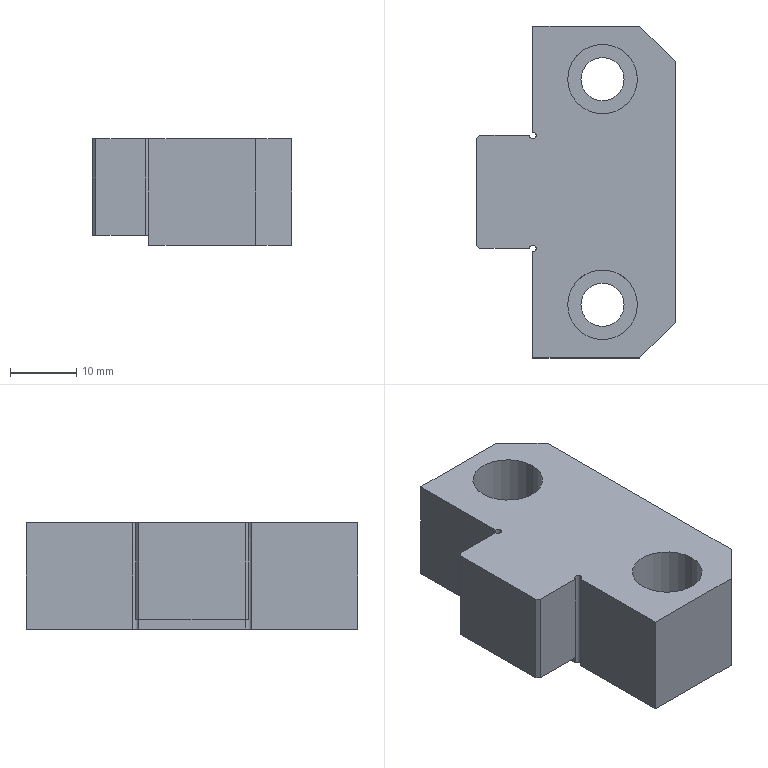Part | STEP file | 2_1 | 1 solid | 28 faces | box 30 x 50 x 16 mm | volume 16891 mm3 | plane 18 | cylinder 10 | commonest cylinder face diameters 6.5 x4 10.5 x4 1 x2